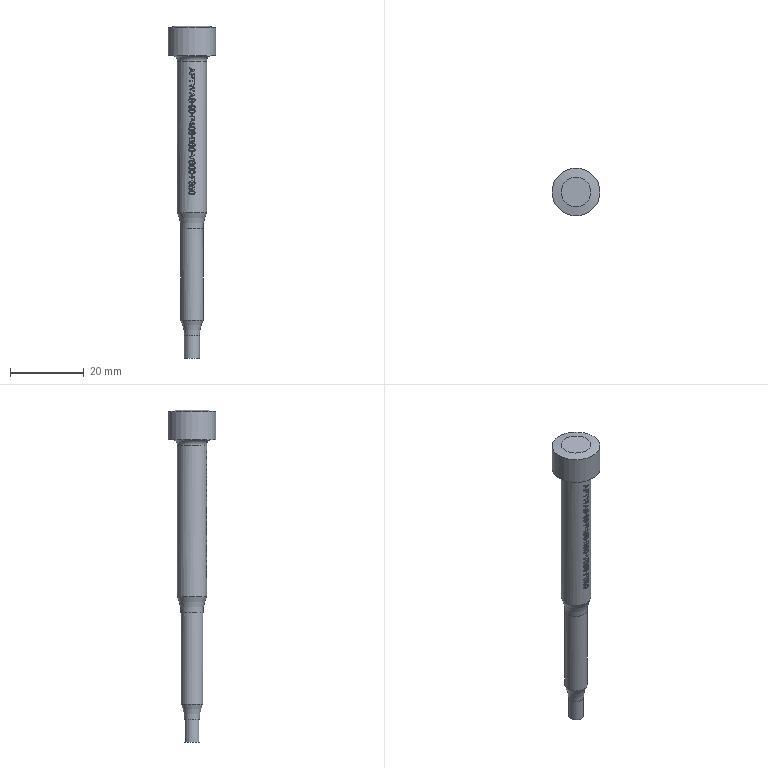Part | NX | features MI_APTWA_0171 2 | 1 solid | 428 faces | box 13 x 13 x 90 mm | volume 4202 mm3 | plane 257 | cylinder 167 | torus 3 | cone 1 | commonest cylinder face diameters 7.8 x32 8 x21 0.687 x6 0.82 x6 0.822 x6 0.832 x6